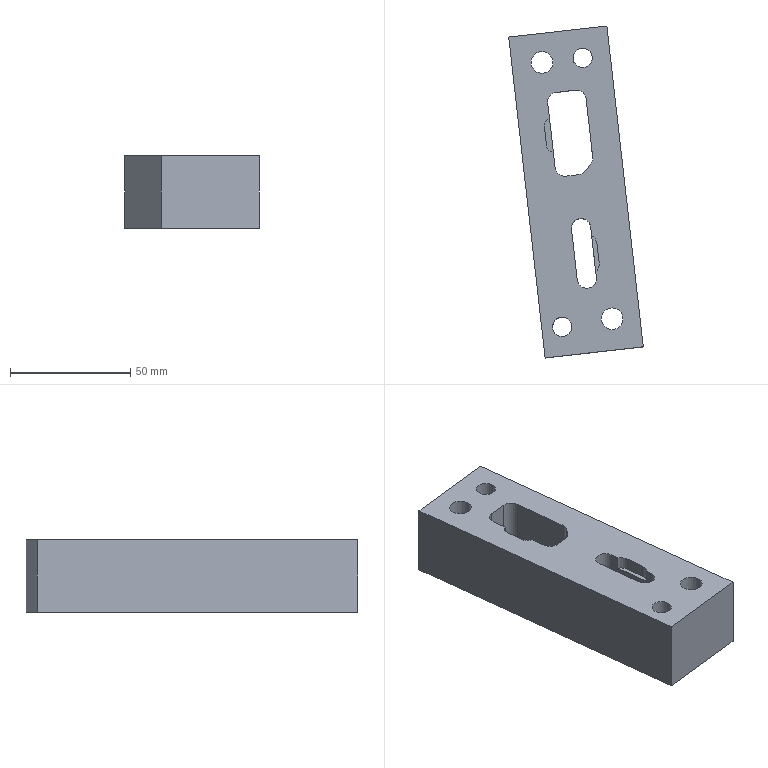Part | NX | features TB 2 | 1 solid | 40 faces | box 55.812 x 137.761 x 30 mm | volume 131881 mm3 | plane 21 | cylinder 19 | commonest cylinder face diameters 8 x7 9 x4 6 x2 8.001 x2 8.5 x2 14.5 x2
STEP:
#1=CARTESIAN_POINT('',(233.25,231.272,30.));
#2=VERTEX_POINT('',#1);
#3=CARTESIAN_POINT('',(233.502,229.054,30.));
#4=VERTEX_POINT('',#3);
#5=CARTESIAN_POINT('',(261.968,-22.421,30.));
#6=DIRECTION('',(0.1125,-0.9937,0.));
#7=VECTOR('',#6,1000.);
#8=LINE('',#5,#7);
#9=EDGE_CURVE('',#2,#4,#8,.T.);
#10=ORIENTED_EDGE('',*,*,#9,.T.);
#11=CARTESIAN_POINT('',(225.552,228.154,30.));
#12=VERTEX_POINT('',#11);
#13=CARTESIAN_POINT('',(229.527,228.604,30.));
#14=DIRECTION('',(0.,0.,1.));
#15=DIRECTION('',(0.,-1.,0.));
#16=AXIS2_PLACEMENT_3D('',#13,#14,#15);
#17=CIRCLE('',#16,4.);
#18=EDGE_CURVE('',#12,#4,#17,.T.);
#19=ORIENTED_EDGE('',*,*,#18,.F.);
#20=CARTESIAN_POINT('',(223.19,249.026,30.));
#21=VERTEX_POINT('',#20);
#22=CARTESIAN_POINT('',(254.019,-23.321,30.));
#23=DIRECTION('',(0.1125,-0.9937,0.));
#24=VECTOR('',#23,1000.);
#25=LINE('',#22,#24);
#26=EDGE_CURVE('',#21,#12,#25,.T.);
#27=ORIENTED_EDGE('',*,*,#26,.F.);
#28=CARTESIAN_POINT('',(231.139,249.926,30.));
#29=VERTEX_POINT('',#28);
#30=CARTESIAN_POINT('',(227.164,249.476,30.));
#31=DIRECTION('',(0.,0.,1.));
#32=DIRECTION('',(0.,-1.,0.));
#33=AXIS2_PLACEMENT_3D('',#30,#31,#32);
#34=CIRCLE('',#33,4.);
#35=EDGE_CURVE('',#29,#21,#34,.T.);
#36=ORIENTED_EDGE('',*,*,#35,.F.);
#37=CARTESIAN_POINT('',(231.527,246.496,30.));
#38=VERTEX_POINT('',#37);
#39=CARTESIAN_POINT('',(261.968,-22.421,30.));
#40=DIRECTION('',(0.1125,-0.9937,0.));
#41=VECTOR('',#40,1000.);
#42=LINE('',#39,#41);
#43=EDGE_CURVE('',#29,#38,#42,.T.);
#44=ORIENTED_EDGE('',*,*,#43,.T.);
#45=CARTESIAN_POINT('',(233.736,243.112,30.));
#46=VERTEX_POINT('',#45);
#47=CARTESIAN_POINT('',(229.265,242.606,30.));
#48=DIRECTION('',(0.,0.,-1.));
#49=DIRECTION('',(0.,-1.,0.));
#50=AXIS2_PLACEMENT_3D('',#47,#48,#49);
#51=CIRCLE('',#50,4.5);
#52=EDGE_CURVE('',#38,#46,#51,.T.);
#53=ORIENTED_EDGE('',*,*,#52,.T.);
#54=CARTESIAN_POINT('',(234.647,235.064,30.));
#55=VERTEX_POINT('',#54);
#56=CARTESIAN_POINT('',(234.372,237.498,30.));
#57=DIRECTION('',(0.1125,-0.9937,0.));
#58=VECTOR('',#57,1000.);
#59=LINE('',#56,#58);
#60=EDGE_CURVE('',#46,#55,#59,.T.);
#61=ORIENTED_EDGE('',*,*,#60,.T.);
#62=CARTESIAN_POINT('',(230.176,234.558,30.));
#63=DIRECTION('',(0.,0.,-1.));
#64=DIRECTION('',(0.,-1.,0.));
#65=AXIS2_PLACEMENT_3D('',#62,#63,#64);
#66=CIRCLE('',#65,4.5);
#67=EDGE_CURVE('',#55,#2,#66,.T.);
#68=ORIENTED_EDGE('',*,*,#67,.T.);
#69=EDGE_LOOP('',(#10,#19,#27,#36,#44,#53,#61,#68));
#70=FACE_BOUND('',#69,.T.);
#71=CARTESIAN_POINT('',(237.879,333.435,30.));
#72=VERTEX_POINT('',#71);
#73=CARTESIAN_POINT('',(252.951,200.285,30.));
#74=VERTEX_POINT('',#73);
#75=CARTESIAN_POINT('',(214.764,537.629,30.));
#76=DIRECTION('',(0.1125,-0.9937,0.));
#77=VECTOR('',#76,1000.);
#78=LINE('',#75,#77);
#79=EDGE_CURVE('',#72,#74,#78,.T.);
#80=ORIENTED_EDGE('',*,*,#79,.F.);
#81=CARTESIAN_POINT('',(197.139,328.823,30.));
#82=VERTEX_POINT('',#81);
#83=CARTESIAN_POINT('',(443.385,356.698,30.));
#84=DIRECTION('',(0.9937,0.1125,0.));
#85=VECTOR('',#84,1000.);
#86=LINE('',#83,#85);
#87=EDGE_CURVE('',#82,#72,#86,.T.);
#88=ORIENTED_EDGE('',*,*,#87,.F.);
#89=CARTESIAN_POINT('',(212.211,195.673,30.));
#90=VERTEX_POINT('',#89);
#91=CARTESIAN_POINT('',(174.024,533.017,30.));
#92=DIRECTION('',(-0.1125,0.9937,0.));
#93=VECTOR('',#92,1000.);
#94=LINE('',#91,#93);
#95=EDGE_CURVE('',#90,#82,#94,.T.);
#96=ORIENTED_EDGE('',*,*,#95,.F.);
#97=CARTESIAN_POINT('',(458.458,223.548,30.));
#98=DIRECTION('',(-0.9937,-0.1125,0.));
#99=VECTOR('',#98,1000.);
#100=LINE('',#97,#99);
#101=EDGE_CURVE('',#74,#90,#100,.T.);
#102=ORIENTED_EDGE('',*,*,#101,.F.);
#103=EDGE_LOOP('',(#80,#88,#96,#102));
#104=FACE_BOUND('',#103,.T.);
#105=CARTESIAN_POINT('',(240.062,216.409,30.));
#106=VERTEX_POINT('',#105);
#107=CARTESIAN_POINT('',(240.062,211.909,30.));
#108=DIRECTION('',(0.,0.,-1.));
#109=DIRECTION('',(0.,1.,0.));
#110=AXIS2_PLACEMENT_3D('',#107,#108,#109);
#111=CIRCLE('',#110,4.5);
#112=EDGE_CURVE('',#106,#106,#111,.T.);
#113=ORIENTED_EDGE('',*,*,#112,.T.);
#114=EDGE_LOOP('',(#113));
#115=FACE_BOUND('',#114,.T.);
#116=CARTESIAN_POINT('',(210.909,322.805,30.));
#117=VERTEX_POINT('',#116);
#118=CARTESIAN_POINT('',(210.909,318.305,30.));
#119=DIRECTION('',(0.,0.,1.));
#120=DIRECTION('',(0.,1.,0.));
#121=AXIS2_PLACEMENT_3D('',#118,#119,#120);
#122=CIRCLE('',#121,4.5);
#123=EDGE_CURVE('',#117,#117,#122,.T.);
#124=ORIENTED_EDGE('',*,*,#123,.F.);
#125=EDGE_LOOP('',(#124));
#126=FACE_BOUND('',#125,.T.);
#127=CARTESIAN_POINT('',(215.619,281.141,30.));
#128=VERTEX_POINT('',#127);
#129=CARTESIAN_POINT('',(212.803,283.799,30.));
#130=VERTEX_POINT('',#129);
#131=CARTESIAN_POINT('',(215.783,284.137,30.));
#132=DIRECTION('',(0.,0.,-1.));
#133=DIRECTION('',(0.,-1.,0.));
#134=AXIS2_PLACEMENT_3D('',#131,#132,#133);
#135=CIRCLE('',#134,3.);
#136=EDGE_CURVE('',#128,#130,#135,.T.);
#137=ORIENTED_EDGE('',*,*,#136,.T.);
#138=CARTESIAN_POINT('',(211.903,291.748,30.));
#139=VERTEX_POINT('',#138);
#140=CARTESIAN_POINT('',(185.72,523.047,30.));
#141=DIRECTION('',(-0.1125,0.9937,0.));
#142=VECTOR('',#141,1000.);
#143=LINE('',#140,#142);
#144=EDGE_CURVE('',#130,#139,#143,.T.);
#145=ORIENTED_EDGE('',*,*,#144,.T.);
#146=CARTESIAN_POINT('',(214.054,294.969,30.));
#147=VERTEX_POINT('',#146);
#148=CARTESIAN_POINT('',(214.884,292.086,30.));
#149=DIRECTION('',(0.,0.,-1.));
#150=DIRECTION('',(0.,-1.,0.));
#151=AXIS2_PLACEMENT_3D('',#148,#149,#150);
#152=CIRCLE('',#151,3.);
#153=EDGE_CURVE('',#139,#147,#152,.T.);
#154=ORIENTED_EDGE('',*,*,#153,.T.);
#155=CARTESIAN_POINT('',(213.318,301.469,30.));
#156=VERTEX_POINT('',#155);
#157=CARTESIAN_POINT('',(186.942,534.48,30.));
#158=DIRECTION('',(0.1125,-0.9937,0.));
#159=VECTOR('',#158,1000.);
#160=LINE('',#157,#159);
#161=EDGE_CURVE('',#156,#147,#160,.T.);
#162=ORIENTED_EDGE('',*,*,#161,.F.);
#163=CARTESIAN_POINT('',(216.843,305.894,30.));
#164=VERTEX_POINT('',#163);
#165=CARTESIAN_POINT('',(217.293,301.919,30.));
#166=DIRECTION('',(0.,0.,1.));
#167=DIRECTION('',(0.,-1.,0.));
#168=AXIS2_PLACEMENT_3D('',#165,#166,#167);
#169=CIRCLE('',#168,4.);
#170=EDGE_CURVE('',#164,#156,#169,.T.);
#171=ORIENTED_EDGE('',*,*,#170,.F.);
#172=CARTESIAN_POINT('',(224.792,306.794,30.));
#173=VERTEX_POINT('',#172);
#174=CARTESIAN_POINT('',(453.153,332.644,30.));
#175=DIRECTION('',(0.9937,0.1125,0.));
#176=VECTOR('',#175,1000.);
#177=LINE('',#174,#176);
#178=EDGE_CURVE('',#164,#173,#177,.T.);
#179=ORIENTED_EDGE('',*,*,#178,.T.);
#180=CARTESIAN_POINT('',(229.217,303.269,30.));
#181=VERTEX_POINT('',#180);
#182=CARTESIAN_POINT('',(225.242,302.819,30.));
#183=DIRECTION('',(0.,0.,1.));
#184=DIRECTION('',(0.,-1.,0.));
#185=AXIS2_PLACEMENT_3D('',#182,#183,#184);
#186=CIRCLE('',#185,4.);
#187=EDGE_CURVE('',#181,#173,#186,.T.);
#188=ORIENTED_EDGE('',*,*,#187,.F.);
#189=CARTESIAN_POINT('',(231.955,279.08,30.));
#190=VERTEX_POINT('',#189);
#191=CARTESIAN_POINT('',(230.585,291.183,30.));
#192=DIRECTION('',(0.1125,-0.9937,0.));
#193=VECTOR('',#192,1000.);
#194=LINE('',#191,#193);
#195=EDGE_CURVE('',#181,#190,#194,.T.);
#196=ORIENTED_EDGE('',*,*,#195,.T.);
#197=CARTESIAN_POINT('',(231.109,276.138,30.));
#198=VERTEX_POINT('',#197);
#199=CARTESIAN_POINT('',(227.98,278.63,30.));
#200=DIRECTION('',(0.,0.,1.));
#201=DIRECTION('',(0.,-1.,0.));
#202=AXIS2_PLACEMENT_3D('',#199,#200,#201);
#203=CIRCLE('',#202,4.);
#204=EDGE_CURVE('',#198,#190,#203,.T.);
#205=ORIENTED_EDGE('',*,*,#204,.F.);
#206=CARTESIAN_POINT('',(228.768,273.199,30.));
#207=VERTEX_POINT('',#206);
#208=CARTESIAN_POINT('',(447.728,548.06,30.));
#209=DIRECTION('',(0.6231,0.7822,0.));
#210=VECTOR('',#209,1000.);
#211=LINE('',#208,#210);
#212=EDGE_CURVE('',#207,#198,#211,.T.);
#213=ORIENTED_EDGE('',*,*,#212,.F.);
#214=CARTESIAN_POINT('',(226.089,271.717,30.));
#215=VERTEX_POINT('',#214);
#216=CARTESIAN_POINT('',(225.639,275.692,30.));
#217=DIRECTION('',(0.,0.,1.));
#218=DIRECTION('',(0.,-1.,0.));
#219=AXIS2_PLACEMENT_3D('',#216,#217,#218);
#220=CIRCLE('',#219,4.);
#221=EDGE_CURVE('',#215,#207,#220,.T.);
#222=ORIENTED_EDGE('',*,*,#221,.F.);
#223=CARTESIAN_POINT('',(220.78,271.116,30.));
#224=VERTEX_POINT('',#223);
#225=CARTESIAN_POINT('',(457.09,297.866,30.));
#226=DIRECTION('',(0.9937,0.1125,0.));
#227=VECTOR('',#226,1000.);
#228=LINE('',#225,#227);
#229=EDGE_CURVE('',#224,#215,#228,.T.);
#230=ORIENTED_EDGE('',*,*,#229,.F.);
#231=CARTESIAN_POINT('',(216.355,274.641,30.));
#232=VERTEX_POINT('',#231);
#233=CARTESIAN_POINT('',(220.33,275.091,30.));
#234=DIRECTION('',(0.,0.,1.));
#235=DIRECTION('',(0.,-1.,0.));
#236=AXIS2_PLACEMENT_3D('',#233,#234,#235);
#237=CIRCLE('',#236,4.);
#238=EDGE_CURVE('',#232,#224,#237,.T.);
#239=ORIENTED_EDGE('',*,*,#238,.F.);
#240=CARTESIAN_POINT('',(186.942,534.48,30.));
#241=DIRECTION('',(0.1125,-0.9937,0.));
#242=VECTOR('',#241,1000.);
#243=LINE('',#240,#242);
#244=EDGE_CURVE('',#128,#232,#243,.T.);
#245=ORIENTED_EDGE('',*,*,#244,.F.);
#246=EDGE_LOOP('',(#137,#145,#154,#162,#171,#179,#188,#196,#205,#213,#222,#230,#239,#245));
#247=FACE_BOUND('',#246,.T.);
#248=CARTESIAN_POINT('',(223.801,320.217,30.));
#249=VERTEX_POINT('',#248);
#250=CARTESIAN_POINT('',(227.801,320.217,30.));
#251=DIRECTION('',(0.,0.,1.));
#252=DIRECTION('',(-1.,0.,0.));
#253=AXIS2_PLACEMENT_3D('',#250,#251,#252);
#254=CIRCLE('',#253,4.);
#255=EDGE_CURVE('',#249,#249,#254,.T.);
#256=ORIENTED_EDGE('',*,*,#255,.F.);
#257=EDGE_LOOP('',(#256));
#258=FACE_BOUND('',#257,.T.);
#259=CARTESIAN_POINT('',(223.308,208.553,30.));
#260=VERTEX_POINT('',#259);
#261=CARTESIAN_POINT('',(219.308,208.553,30.));
#262=DIRECTION('',(0.,0.,-1.));
#263=DIRECTION('',(1.,0.,0.));
#264=AXIS2_PLACEMENT_3D('',#261,#262,#263);
#265=CIRCLE('',#264,4.);
#266=EDGE_CURVE('',#260,#260,#265,.T.);
#267=ORIENTED_EDGE('',*,*,#266,.T.);
#268=EDGE_LOOP('',(#267));
#269=FACE_BOUND('',#268,.T.);
#270=CARTESIAN_POINT('',(427.226,561.68,30.));
#271=DIRECTION('',(0.,0.,-1.));
#272=DIRECTION('',(-0.9981,0.06177,0.));
#273=AXIS2_PLACEMENT_3D('',#270,#271,#272);
#274=PLANE('',#273);
#275=ADVANCED_FACE('',(#70,#104,#115,#126,#247,#258,#269),#274,.F.);
#276=CARTESIAN_POINT('',(219.308,204.303,0.));
#277=VERTEX_POINT('',#276);
#278=CARTESIAN_POINT('',(219.308,208.553,0.));
#279=DIRECTION('',(0.,0.,1.));
#280=DIRECTION('',(0.,-1.,0.));
#281=AXIS2_PLACEMENT_3D('',#278,#279,#280);
#282=CIRCLE('',#281,4.25);
#283=EDGE_CURVE('',#277,#277,#282,.T.);
#284=ORIENTED_EDGE('',*,*,#283,.T.);
#285=EDGE_LOOP('',(#284));
#286=FACE_BOUND('',#285,.T.);
#287=CARTESIAN_POINT('',(227.801,315.967,0.));
#288=VERTEX_POINT('',#287);
#289=CARTESIAN_POINT('',(227.801,320.217,0.));
#290=DIRECTION('',(0.,0.,1.));
#291=DIRECTION('',(0.,-1.,0.));
#292=AXIS2_PLACEMENT_3D('',#289,#290,#291);
#293=CIRCLE('',#292,4.25);
#294=EDGE_CURVE('',#288,#288,#293,.T.);
#295=ORIENTED_EDGE('',*,*,#294,.T.);
#296=EDGE_LOOP('',(#295));
#297=FACE_BOUND('',#296,.T.);
#298=CARTESIAN_POINT('',(231.955,279.08,0.));
#299=VERTEX_POINT('',#298);
#300=CARTESIAN_POINT('',(229.217,303.269,0.));
#301=VERTEX_POINT('',#300);
#302=CARTESIAN_POINT('',(230.585,291.183,0.));
#303=DIRECTION('',(-0.1125,0.9937,0.));
#304=VECTOR('',#303,1000.);
#305=LINE('',#302,#304);
#306=EDGE_CURVE('',#299,#301,#305,.T.);
#307=ORIENTED_EDGE('',*,*,#306,.T.);
#308=CARTESIAN_POINT('',(224.792,306.794,0.));
#309=VERTEX_POINT('',#308);
#310=CARTESIAN_POINT('',(225.242,302.819,0.));
#311=DIRECTION('',(0.,0.,-1.));
#312=DIRECTION('',(0.,-1.,0.));
#313=AXIS2_PLACEMENT_3D('',#310,#311,#312);
#314=CIRCLE('',#313,4.);
#315=EDGE_CURVE('',#309,#301,#314,.T.);
#316=ORIENTED_EDGE('',*,*,#315,.F.);
#317=CARTESIAN_POINT('',(216.843,305.894,0.));
#318=VERTEX_POINT('',#317);
#319=CARTESIAN_POINT('',(453.153,332.644,0.));
#320=DIRECTION('',(-0.9937,-0.1125,0.));
#321=VECTOR('',#320,1000.);
#322=LINE('',#319,#321);
#323=EDGE_CURVE('',#309,#318,#322,.T.);
#324=ORIENTED_EDGE('',*,*,#323,.T.);
#325=CARTESIAN_POINT('',(213.318,301.469,0.));
#326=VERTEX_POINT('',#325);
#327=CARTESIAN_POINT('',(217.293,301.919,0.));
#328=DIRECTION('',(0.,0.,-1.));
#329=DIRECTION('',(0.,-1.,0.));
#330=AXIS2_PLACEMENT_3D('',#327,#328,#329);
#331=CIRCLE('',#330,4.);
#332=EDGE_CURVE('',#326,#318,#331,.T.);
#333=ORIENTED_EDGE('',*,*,#332,.F.);
#334=CARTESIAN_POINT('',(216.355,274.641,0.));
#335=VERTEX_POINT('',#334);
#336=CARTESIAN_POINT('',(214.837,288.055,0.));
#337=DIRECTION('',(0.1125,-0.9937,0.));
#338=VECTOR('',#337,1000.);
#339=LINE('',#336,#338);
#340=EDGE_CURVE('',#326,#335,#339,.T.);
#341=ORIENTED_EDGE('',*,*,#340,.T.);
#342=CARTESIAN_POINT('',(220.78,271.116,0.));
#343=VERTEX_POINT('',#342);
#344=CARTESIAN_POINT('',(220.33,275.091,0.));
#345=DIRECTION('',(0.,0.,-1.));
#346=DIRECTION('',(0.,-1.,0.));
#347=AXIS2_PLACEMENT_3D('',#344,#345,#346);
#348=CIRCLE('',#347,4.);
#349=EDGE_CURVE('',#343,#335,#348,.T.);
#350=ORIENTED_EDGE('',*,*,#349,.F.);
#351=CARTESIAN_POINT('',(226.089,271.717,0.));
#352=VERTEX_POINT('',#351);
#353=CARTESIAN_POINT('',(457.09,297.866,0.));
#354=DIRECTION('',(-0.9937,-0.1125,0.));
#355=VECTOR('',#354,1000.);
#356=LINE('',#353,#355);
#357=EDGE_CURVE('',#352,#343,#356,.T.);
#358=ORIENTED_EDGE('',*,*,#357,.F.);
#359=CARTESIAN_POINT('',(228.768,273.199,0.));
#360=VERTEX_POINT('',#359);
#361=CARTESIAN_POINT('',(225.639,275.692,0.));
#362=DIRECTION('',(0.,0.,-1.));
#363=DIRECTION('',(0.,-1.,0.));
#364=AXIS2_PLACEMENT_3D('',#361,#362,#363);
#365=CIRCLE('',#364,4.);
#366=EDGE_CURVE('',#360,#352,#365,.T.);
#367=ORIENTED_EDGE('',*,*,#366,.F.);
#368=CARTESIAN_POINT('',(231.109,276.138,0.));
#369=VERTEX_POINT('',#368);
#370=CARTESIAN_POINT('',(447.728,548.06,0.));
#371=DIRECTION('',(-0.6231,-0.7822,0.));
#372=VECTOR('',#371,1000.);
#373=LINE('',#370,#372);
#374=EDGE_CURVE('',#369,#360,#373,.T.);
#375=ORIENTED_EDGE('',*,*,#374,.F.);
#376=CARTESIAN_POINT('',(227.98,278.63,0.));
#377=DIRECTION('',(0.,0.,-1.));
#378=DIRECTION('',(0.,-1.,0.));
#379=AXIS2_PLACEMENT_3D('',#376,#377,#378);
#380=CIRCLE('',#379,4.);
#381=EDGE_CURVE('',#299,#369,#380,.T.);
#382=ORIENTED_EDGE('',*,*,#381,.F.);
#383=EDGE_LOOP('',(#307,#316,#324,#333,#341,#350,#358,#367,#375,#382));
#384=FACE_BOUND('',#383,.T.);
#385=CARTESIAN_POINT('',(231.139,249.926,0.));
#386=VERTEX_POINT('',#385);
#387=CARTESIAN_POINT('',(233.502,229.054,0.));
#388=VERTEX_POINT('',#387);
#389=CARTESIAN_POINT('',(261.968,-22.421,0.));
#390=DIRECTION('',(0.1125,-0.9937,0.));
#391=VECTOR('',#390,1000.);
#392=LINE('',#389,#391);
#393=EDGE_CURVE('',#386,#388,#392,.T.);
#394=ORIENTED_EDGE('',*,*,#393,.F.);
#395=CARTESIAN_POINT('',(223.19,249.026,0.));
#396=VERTEX_POINT('',#395);
#397=CARTESIAN_POINT('',(227.164,249.476,0.));
#398=DIRECTION('',(0.,0.,-1.));
#399=DIRECTION('',(0.,-1.,0.));
#400=AXIS2_PLACEMENT_3D('',#397,#398,#399);
#401=CIRCLE('',#400,4.);
#402=EDGE_CURVE('',#396,#386,#401,.T.);
#403=ORIENTED_EDGE('',*,*,#402,.F.);
#404=CARTESIAN_POINT('',(225.552,228.154,0.));
#405=VERTEX_POINT('',#404);
#406=CARTESIAN_POINT('',(225.777,226.166,0.));
#407=DIRECTION('',(-0.1125,0.9937,0.));
#408=VECTOR('',#407,1000.);
#409=LINE('',#406,#408);
#410=EDGE_CURVE('',#405,#396,#409,.T.);
#411=ORIENTED_EDGE('',*,*,#410,.F.);
#412=CARTESIAN_POINT('',(229.527,228.604,0.));
#413=DIRECTION('',(0.,0.,-1.));
#414=DIRECTION('',(0.,-1.,0.));
#415=AXIS2_PLACEMENT_3D('',#412,#413,#414);
#416=CIRCLE('',#415,4.);
#417=EDGE_CURVE('',#388,#405,#416,.T.);
#418=ORIENTED_EDGE('',*,*,#417,.F.);
#419=EDGE_LOOP('',(#394,#403,#411,#418));
#420=FACE_BOUND('',#419,.T.);
#421=CARTESIAN_POINT('',(210.909,325.555,0.));
#422=VERTEX_POINT('',#421);
#423=CARTESIAN_POINT('',(210.909,318.305,0.));
#424=DIRECTION('',(0.,0.,1.));
#425=DIRECTION('',(0.,1.,0.));
#426=AXIS2_PLACEMENT_3D('',#423,#424,#425);
#427=CIRCLE('',#426,7.25);
#428=EDGE_CURVE('',#422,#422,#427,.T.);
#429=ORIENTED_EDGE('',*,*,#428,.T.);
#430=EDGE_LOOP('',(#429));
#431=FACE_BOUND('',#430,.T.);
#432=CARTESIAN_POINT('',(240.062,219.159,0.));
#433=VERTEX_POINT('',#432);
#434=CARTESIAN_POINT('',(240.062,211.909,0.));
#435=DIRECTION('',(0.,0.,-1.));
#436=DIRECTION('',(0.,1.,0.));
#437=AXIS2_PLACEMENT_3D('',#434,#435,#436);
#438=CIRCLE('',#437,7.25);
#439=EDGE_CURVE('',#433,#433,#438,.T.);
#440=ORIENTED_EDGE('',*,*,#439,.F.);
#441=EDGE_LOOP('',(#440));
#442=FACE_BOUND('',#441,.T.);
#443=CARTESIAN_POINT('',(197.139,328.823,0.));
#444=VERTEX_POINT('',#443);
#445=CARTESIAN_POINT('',(237.879,333.435,0.));
#446=VERTEX_POINT('',#445);
#447=CARTESIAN_POINT('',(443.385,356.698,0.));
#448=DIRECTION('',(0.9937,0.1125,0.));
#449=VECTOR('',#448,1000.);
#450=LINE('',#447,#449);
#451=EDGE_CURVE('',#444,#446,#450,.T.);
#452=ORIENTED_EDGE('',*,*,#451,.T.);
#453=CARTESIAN_POINT('',(252.951,200.285,0.));
#454=VERTEX_POINT('',#453);
#455=CARTESIAN_POINT('',(214.764,537.629,0.));
#456=DIRECTION('',(0.1125,-0.9937,0.));
#457=VECTOR('',#456,1000.);
#458=LINE('',#455,#457);
#459=EDGE_CURVE('',#446,#454,#458,.T.);
#460=ORIENTED_EDGE('',*,*,#459,.T.);
#461=CARTESIAN_POINT('',(212.211,195.673,0.));
#462=VERTEX_POINT('',#461);
#463=CARTESIAN_POINT('',(458.458,223.548,0.));
#464=DIRECTION('',(-0.9937,-0.1125,0.));
#465=VECTOR('',#464,1000.);
#466=LINE('',#463,#465);
#467=EDGE_CURVE('',#454,#462,#466,.T.);
#468=ORIENTED_EDGE('',*,*,#467,.T.);
#469=CARTESIAN_POINT('',(174.024,533.017,0.));
#470=DIRECTION('',(-0.1125,0.9937,0.));
#471=VECTOR('',#470,1000.);
#472=LINE('',#469,#471);
#473=EDGE_CURVE('',#462,#444,#472,.T.);
#474=ORIENTED_EDGE('',*,*,#473,.T.);
#475=EDGE_LOOP('',(#452,#460,#468,#474));
#476=FACE_BOUND('',#475,.T.);
#477=CARTESIAN_POINT('',(420.271,560.892,0.));
#478=DIRECTION('',(0.,0.,-1.));
#479=DIRECTION('',(-0.9981,0.06177,0.));
#480=AXIS2_PLACEMENT_3D('',#477,#478,#479);
#481=PLANE('',#480);
#482=ADVANCED_FACE('',(#286,#297,#384,#420,#431,#442,#476),#481,.T.);
#483=CARTESIAN_POINT('',(233.25,231.272,24.8));
#484=VERTEX_POINT('',#483);
#485=CARTESIAN_POINT('',(234.647,235.064,24.8));
#486=VERTEX_POINT('',#485);
#487=CARTESIAN_POINT('',(230.176,234.558,24.8));
#488=DIRECTION('',(0.,0.,1.));
#489=DIRECTION('',(0.,1.,0.));
#490=AXIS2_PLACEMENT_3D('',#487,#488,#489);
#491=CIRCLE('',#490,4.5);
#492=EDGE_CURVE('',#484,#486,#491,.T.);
#493=ORIENTED_EDGE('',*,*,#492,.T.);
#494=CARTESIAN_POINT('',(233.736,243.112,24.8));
#495=VERTEX_POINT('',#494);
#496=CARTESIAN_POINT('',(234.372,237.498,24.8));
#497=DIRECTION('',(0.1125,-0.9937,0.));
#498=VECTOR('',#497,1000.);
#499=LINE('',#496,#498);
#500=EDGE_CURVE('',#495,#486,#499,.T.);
#501=ORIENTED_EDGE('',*,*,#500,.F.);
#502=CARTESIAN_POINT('',(231.527,246.496,24.8));
#503=VERTEX_POINT('',#502);
#504=CARTESIAN_POINT('',(229.265,242.606,24.8));
#505=DIRECTION('',(0.,0.,1.));
#506=DIRECTION('',(0.,1.,0.));
#507=AXIS2_PLACEMENT_3D('',#504,#505,#506);
#508=CIRCLE('',#507,4.5);
#509=EDGE_CURVE('',#495,#503,#508,.T.);
#510=ORIENTED_EDGE('',*,*,#509,.T.);
#511=CARTESIAN_POINT('',(233.727,227.066,24.8));
#512=DIRECTION('',(-0.1125,0.9937,0.));
#513=VECTOR('',#512,1000.);
#514=LINE('',#511,#513);
#515=EDGE_CURVE('',#484,#503,#514,.T.);
#516=ORIENTED_EDGE('',*,*,#515,.F.);
#517=EDGE_LOOP('',(#493,#501,#510,#516));
#518=FACE_BOUND('',#517,.T.);
#519=CARTESIAN_POINT('',(223.64,236.283,24.8));
#520=DIRECTION('',(0.,0.,-1.));
#521=DIRECTION('',(-0.9981,0.06177,0.));
#522=AXIS2_PLACEMENT_3D('',#519,#520,#521);
#523=PLANE('',#522);
#524=ADVANCED_FACE('',(#518),#523,.F.);
#525=ORIENTED_EDGE('',*,*,#509,.F.);
#526=CARTESIAN_POINT('',(233.736,243.112,25.7));
#527=DIRECTION('',(0.,0.,-1.));
#528=VECTOR('',#527,1000.);
#529=LINE('',#526,#528);
#530=EDGE_CURVE('',#46,#495,#529,.T.);
#531=ORIENTED_EDGE('',*,*,#530,.F.);
#532=ORIENTED_EDGE('',*,*,#52,.F.);
#533=CARTESIAN_POINT('',(231.527,246.496,25.7));
#534=DIRECTION('',(0.,0.,1.));
#535=VECTOR('',#534,1000.);
#536=LINE('',#533,#535);
#537=EDGE_CURVE('',#503,#38,#536,.T.);
#538=ORIENTED_EDGE('',*,*,#537,.F.);
#539=EDGE_LOOP('',(#525,#531,#532,#538));
#540=FACE_BOUND('',#539,.T.);
#541=CARTESIAN_POINT('',(229.265,242.606,25.7));
#542=DIRECTION('',(0.,0.,1.));
#543=DIRECTION('',(0.9981,-0.06177,0.));
#544=AXIS2_PLACEMENT_3D('',#541,#542,#543);
#545=CYLINDRICAL_SURFACE('',#544,4.5);
#546=ADVANCED_FACE('',(#540),#545,.F.);
#547=ORIENTED_EDGE('',*,*,#67,.F.);
#548=CARTESIAN_POINT('',(234.647,235.064,25.7));
#549=DIRECTION('',(0.,0.,1.));
#550=VECTOR('',#549,1000.);
#551=LINE('',#548,#550);
#552=EDGE_CURVE('',#486,#55,#551,.T.);
#553=ORIENTED_EDGE('',*,*,#552,.F.);
#554=ORIENTED_EDGE('',*,*,#492,.F.);
#555=CARTESIAN_POINT('',(233.25,231.272,25.7));
#556=DIRECTION('',(0.,0.,-1.));
#557=VECTOR('',#556,1000.);
#558=LINE('',#555,#557);
#559=EDGE_CURVE('',#2,#484,#558,.T.);
#560=ORIENTED_EDGE('',*,*,#559,.F.);
#561=EDGE_LOOP('',(#547,#553,#554,#560));
#562=FACE_BOUND('',#561,.T.);
#563=CARTESIAN_POINT('',(230.176,234.558,25.7));
#564=DIRECTION('',(0.,0.,1.));
#565=DIRECTION('',(0.9981,-0.06177,0.));
#566=AXIS2_PLACEMENT_3D('',#563,#564,#565);
#567=CYLINDRICAL_SURFACE('',#566,4.5);
#568=ADVANCED_FACE('',(#562),#567,.F.);
#569=CARTESIAN_POINT('',(215.619,281.141,24.8));
#570=VERTEX_POINT('',#569);
#571=CARTESIAN_POINT('',(214.054,294.969,24.8));
#572=VERTEX_POINT('',#571);
#573=CARTESIAN_POINT('',(213.993,295.507,24.8));
#574=DIRECTION('',(-0.1125,0.9937,0.));
#575=VECTOR('',#574,1000.);
#576=LINE('',#573,#575);
#577=EDGE_CURVE('',#570,#572,#576,.T.);
#578=ORIENTED_EDGE('',*,*,#577,.T.);
#579=CARTESIAN_POINT('',(211.903,291.748,24.8));
#580=VERTEX_POINT('',#579);
#581=CARTESIAN_POINT('',(214.884,292.086,24.8));
#582=DIRECTION('',(0.,0.,1.));
#583=DIRECTION('',(-0.9981,0.06177,0.));
#584=AXIS2_PLACEMENT_3D('',#581,#582,#583);
#585=CIRCLE('',#584,3.);
#586=EDGE_CURVE('',#572,#580,#585,.T.);
#587=ORIENTED_EDGE('',*,*,#586,.T.);
#588=CARTESIAN_POINT('',(212.803,283.799,24.8));
#589=VERTEX_POINT('',#588);
#590=CARTESIAN_POINT('',(185.72,523.047,24.8));
#591=DIRECTION('',(-0.1125,0.9937,0.));
#592=VECTOR('',#591,1000.);
#593=LINE('',#590,#592);
#594=EDGE_CURVE('',#589,#580,#593,.T.);
#595=ORIENTED_EDGE('',*,*,#594,.F.);
#596=CARTESIAN_POINT('',(215.783,284.137,24.8));
#597=DIRECTION('',(0.,0.,1.));
#598=DIRECTION('',(-0.9981,0.06177,0.));
#599=AXIS2_PLACEMENT_3D('',#596,#597,#598);
#600=CIRCLE('',#599,3.);
#601=EDGE_CURVE('',#589,#570,#600,.T.);
#602=ORIENTED_EDGE('',*,*,#601,.T.);
#603=EDGE_LOOP('',(#578,#587,#595,#602));
#604=FACE_BOUND('',#603,.T.);
#605=CARTESIAN_POINT('',(213.496,295.451,24.8));
#606=DIRECTION('',(0.,0.,1.));
#607=DIRECTION('',(-0.9981,0.06177,0.));
#608=AXIS2_PLACEMENT_3D('',#605,#606,#607);
#609=PLANE('',#608);
#610=ADVANCED_FACE('',(#604),#609,.T.);
#611=CARTESIAN_POINT('',(240.062,219.159,15.));
#612=VERTEX_POINT('',#611);
#613=CARTESIAN_POINT('',(240.062,211.909,15.));
#614=DIRECTION('',(0.,0.,1.));
#615=DIRECTION('',(0.,1.,0.));
#616=AXIS2_PLACEMENT_3D('',#613,#614,#615);
#617=CIRCLE('',#616,7.25);
#618=EDGE_CURVE('',#612,#612,#617,.T.);
#619=ORIENTED_EDGE('',*,*,#618,.F.);
#620=EDGE_LOOP('',(#619));
#621=FACE_BOUND('',#620,.T.);
#622=CARTESIAN_POINT('',(240.062,216.409,15.));
#623=VERTEX_POINT('',#622);
#624=CARTESIAN_POINT('',(240.062,211.909,15.));
#625=DIRECTION('',(0.,0.,-1.));
#626=DIRECTION('',(0.,1.,0.));
#627=AXIS2_PLACEMENT_3D('',#624,#625,#626);
#628=CIRCLE('',#627,4.5);
#629=EDGE_CURVE('',#623,#623,#628,.T.);
#630=ORIENTED_EDGE('',*,*,#629,.F.);
#631=EDGE_LOOP('',(#630));
#632=FACE_BOUND('',#631,.T.);
#633=CARTESIAN_POINT('',(220.808,284.202,15.));
#634=DIRECTION('',(0.,0.,-1.));
#635=DIRECTION('',(0.9981,-0.06177,0.));
#636=AXIS2_PLACEMENT_3D('',#633,#634,#635);
#637=PLANE('',#636);
#638=ADVANCED_FACE('',(#621,#632),#637,.T.);
#639=CARTESIAN_POINT('',(210.909,322.805,15.));
#640=VERTEX_POINT('',#639);
#641=CARTESIAN_POINT('',(210.909,318.305,15.));
#642=DIRECTION('',(0.,0.,1.));
#643=DIRECTION('',(0.,1.,0.));
#644=AXIS2_PLACEMENT_3D('',#641,#642,#643);
#645=CIRCLE('',#644,4.5);
#646=EDGE_CURVE('',#640,#640,#645,.T.);
#647=ORIENTED_EDGE('',*,*,#646,.T.);
#648=EDGE_LOOP('',(#647));
#649=FACE_BOUND('',#648,.T.);
#650=CARTESIAN_POINT('',(210.909,325.555,15.));
#651=VERTEX_POINT('',#650);
#652=CARTESIAN_POINT('',(210.909,318.305,15.));
#653=DIRECTION('',(0.,0.,-1.));
#654=DIRECTION('',(0.,1.,0.));
#655=AXIS2_PLACEMENT_3D('',#652,#653,#654);
#656=CIRCLE('',#655,7.25);
#657=EDGE_CURVE('',#651,#651,#656,.T.);
#658=ORIENTED_EDGE('',*,*,#657,.T.);
#659=EDGE_LOOP('',(#658));
#660=FACE_BOUND('',#659,.T.);
#661=CARTESIAN_POINT('',(220.808,284.202,15.));
#662=DIRECTION('',(0.,0.,-1.));
#663=DIRECTION('',(0.9981,-0.06177,0.));
#664=AXIS2_PLACEMENT_3D('',#661,#662,#663);
#665=PLANE('',#664);
#666=ADVANCED_FACE('',(#649,#660),#665,.T.);
#667=ORIENTED_EDGE('',*,*,#123,.T.);
#668=EDGE_LOOP('',(#667));
#669=FACE_BOUND('',#668,.T.);
#670=ORIENTED_EDGE('',*,*,#646,.F.);
#671=EDGE_LOOP('',(#670));
#672=FACE_BOUND('',#671,.T.);
#673=CARTESIAN_POINT('',(210.909,318.305,15.));
#674=DIRECTION('',(0.,0.,1.));
#675=DIRECTION('',(-0.9981,0.06177,0.));
#676=AXIS2_PLACEMENT_3D('',#673,#674,#675);
#677=CYLINDRICAL_SURFACE('',#676,4.5);
#678=ADVANCED_FACE('',(#669,#672),#677,.F.);
#679=ORIENTED_EDGE('',*,*,#112,.F.);
#680=EDGE_LOOP('',(#679));
#681=FACE_BOUND('',#680,.T.);
#682=ORIENTED_EDGE('',*,*,#629,.T.);
#683=EDGE_LOOP('',(#682));
#684=FACE_BOUND('',#683,.T.);
#685=CARTESIAN_POINT('',(240.062,211.909,15.));
#686=DIRECTION('',(0.,0.,-1.));
#687=DIRECTION('',(0.9981,-0.06177,0.));
#688=AXIS2_PLACEMENT_3D('',#685,#686,#687);
#689=CYLINDRICAL_SURFACE('',#688,4.5);
#690=ADVANCED_FACE('',(#681,#684),#689,.F.);
#691=ORIENTED_EDGE('',*,*,#153,.F.);
#692=CARTESIAN_POINT('',(211.903,291.748,14.5));
#693=DIRECTION('',(0.,0.,1.));
#694=VECTOR('',#693,1000.);
#695=LINE('',#692,#694);
#696=EDGE_CURVE('',#580,#139,#695,.T.);
#697=ORIENTED_EDGE('',*,*,#696,.F.);
#698=ORIENTED_EDGE('',*,*,#586,.F.);
#699=CARTESIAN_POINT('',(214.054,294.969,14.5));
#700=DIRECTION('',(0.,0.,-1.));
#701=VECTOR('',#700,1000.);
#702=LINE('',#699,#701);
#703=EDGE_CURVE('',#147,#572,#702,.T.);
#704=ORIENTED_EDGE('',*,*,#703,.F.);
#705=EDGE_LOOP('',(#691,#697,#698,#704));
#706=FACE_BOUND('',#705,.T.);
#707=CARTESIAN_POINT('',(214.884,292.086,14.5));
#708=DIRECTION('',(0.,0.,1.));
#709=DIRECTION('',(-0.9981,0.06177,0.));
#710=AXIS2_PLACEMENT_3D('',#707,#708,#709);
#711=CYLINDRICAL_SURFACE('',#710,3.);
#712=ADVANCED_FACE('',(#706),#711,.F.);
#713=ORIENTED_EDGE('',*,*,#594,.T.);
#714=ORIENTED_EDGE('',*,*,#696,.T.);
#715=ORIENTED_EDGE('',*,*,#144,.F.);
#716=CARTESIAN_POINT('',(212.803,283.799,14.5));
#717=DIRECTION('',(0.,0.,-1.));
#718=VECTOR('',#717,1000.);
#719=LINE('',#716,#718);
#720=EDGE_CURVE('',#130,#589,#719,.T.);
#721=ORIENTED_EDGE('',*,*,#720,.T.);
#722=EDGE_LOOP('',(#713,#714,#715,#721));
#723=FACE_BOUND('',#722,.T.);
#724=CARTESIAN_POINT('',(185.72,523.047,14.5));
#725=DIRECTION('',(-0.9937,-0.1125,0.));
#726=DIRECTION('',(0.1125,-0.9937,0.));
#727=AXIS2_PLACEMENT_3D('',#724,#725,#726);
#728=PLANE('',#727);
#729=ADVANCED_FACE('',(#723),#728,.F.);
#730=ORIENTED_EDGE('',*,*,#601,.F.);
#731=ORIENTED_EDGE('',*,*,#720,.F.);
#732=ORIENTED_EDGE('',*,*,#136,.F.);
#733=CARTESIAN_POINT('',(215.619,281.141,14.5));
#734=DIRECTION('',(0.,0.,1.));
#735=VECTOR('',#734,1000.);
#736=LINE('',#733,#735);
#737=EDGE_CURVE('',#570,#128,#736,.T.);
#738=ORIENTED_EDGE('',*,*,#737,.F.);
#739=EDGE_LOOP('',(#730,#731,#732,#738));
#740=FACE_BOUND('',#739,.T.);
#741=CARTESIAN_POINT('',(215.783,284.137,14.5));
#742=DIRECTION('',(0.,0.,-1.));
#743=DIRECTION('',(0.9981,-0.06177,0.));
#744=AXIS2_PLACEMENT_3D('',#741,#742,#743);
#745=CYLINDRICAL_SURFACE('',#744,3.);
#746=ADVANCED_FACE('',(#740),#745,.F.);
#747=ORIENTED_EDGE('',*,*,#95,.T.);
#748=CARTESIAN_POINT('',(197.139,328.823,0.));
#749=DIRECTION('',(0.,0.,1.));
#750=VECTOR('',#749,1000.);
#751=LINE('',#748,#750);
#752=EDGE_CURVE('',#444,#82,#751,.T.);
#753=ORIENTED_EDGE('',*,*,#752,.F.);
#754=ORIENTED_EDGE('',*,*,#473,.F.);
#755=CARTESIAN_POINT('',(212.211,195.673,0.));
#756=DIRECTION('',(0.,0.,1.));
#757=VECTOR('',#756,1000.);
#758=LINE('',#755,#757);
#759=EDGE_CURVE('',#462,#90,#758,.T.);
#760=ORIENTED_EDGE('',*,*,#759,.T.);
#761=EDGE_LOOP('',(#747,#753,#754,#760));
#762=FACE_BOUND('',#761,.T.);
#763=CARTESIAN_POINT('',(174.024,533.017,0.));
#764=DIRECTION('',(-0.9937,-0.1125,0.));
#765=DIRECTION('',(-0.1125,0.9937,0.));
#766=AXIS2_PLACEMENT_3D('',#763,#764,#765);
#767=PLANE('',#766);
#768=ADVANCED_FACE('',(#762),#767,.T.);
#769=ORIENTED_EDGE('',*,*,#467,.F.);
#770=CARTESIAN_POINT('',(252.951,200.285,0.));
#771=DIRECTION('',(0.,0.,1.));
#772=VECTOR('',#771,1000.);
#773=LINE('',#770,#772);
#774=EDGE_CURVE('',#454,#74,#773,.T.);
#775=ORIENTED_EDGE('',*,*,#774,.T.);
#776=ORIENTED_EDGE('',*,*,#101,.T.);
#777=ORIENTED_EDGE('',*,*,#759,.F.);
#778=EDGE_LOOP('',(#769,#775,#776,#777));
#779=FACE_BOUND('',#778,.T.);
#780=CARTESIAN_POINT('',(458.458,223.548,0.));
#781=DIRECTION('',(0.1125,-0.9937,0.));
#782=DIRECTION('',(-0.9937,-0.1125,0.));
#783=AXIS2_PLACEMENT_3D('',#780,#781,#782);
#784=PLANE('',#783);
#785=ADVANCED_FACE('',(#779),#784,.T.);
#786=ORIENTED_EDGE('',*,*,#459,.F.);
#787=CARTESIAN_POINT('',(237.879,333.435,0.));
#788=DIRECTION('',(0.,0.,1.));
#789=VECTOR('',#788,1000.);
#790=LINE('',#787,#789);
#791=EDGE_CURVE('',#446,#72,#790,.T.);
#792=ORIENTED_EDGE('',*,*,#791,.T.);
#793=ORIENTED_EDGE('',*,*,#79,.T.);
#794=ORIENTED_EDGE('',*,*,#774,.F.);
#795=EDGE_LOOP('',(#786,#792,#793,#794));
#796=FACE_BOUND('',#795,.T.);
#797=CARTESIAN_POINT('',(214.764,537.629,0.));
#798=DIRECTION('',(0.9937,0.1125,0.));
#799=DIRECTION('',(0.1125,-0.9937,0.));
#800=AXIS2_PLACEMENT_3D('',#797,#798,#799);
#801=PLANE('',#800);
#802=ADVANCED_FACE('',(#796),#801,.T.);
#803=ORIENTED_EDGE('',*,*,#87,.T.);
#804=ORIENTED_EDGE('',*,*,#791,.F.);
#805=ORIENTED_EDGE('',*,*,#451,.F.);
#806=ORIENTED_EDGE('',*,*,#752,.T.);
#807=EDGE_LOOP('',(#803,#804,#805,#806));
#808=FACE_BOUND('',#807,.T.);
#809=CARTESIAN_POINT('',(443.385,356.698,0.));
#810=DIRECTION('',(-0.1125,0.9937,0.));
#811=DIRECTION('',(0.9937,0.1125,0.));
#812=AXIS2_PLACEMENT_3D('',#809,#810,#811);
#813=PLANE('',#812);
#814=ADVANCED_FACE('',(#808),#813,.T.);
#815=ORIENTED_EDGE('',*,*,#618,.T.);
#816=EDGE_LOOP('',(#815));
#817=FACE_BOUND('',#816,.T.);
#818=ORIENTED_EDGE('',*,*,#439,.T.);
#819=EDGE_LOOP('',(#818));
#820=FACE_BOUND('',#819,.T.);
#821=CARTESIAN_POINT('',(240.062,211.909,0.));
#822=DIRECTION('',(0.,0.,-1.));
#823=DIRECTION('',(0.9981,-0.06177,0.));
#824=AXIS2_PLACEMENT_3D('',#821,#822,#823);
#825=CYLINDRICAL_SURFACE('',#824,7.25);
#826=ADVANCED_FACE('',(#817,#820),#825,.F.);
#827=ORIENTED_EDGE('',*,*,#657,.F.);
#828=EDGE_LOOP('',(#827));
#829=FACE_BOUND('',#828,.T.);
#830=ORIENTED_EDGE('',*,*,#428,.F.);
#831=EDGE_LOOP('',(#830));
#832=FACE_BOUND('',#831,.T.);
#833=CARTESIAN_POINT('',(210.909,318.305,0.));
#834=DIRECTION('',(0.,0.,1.));
#835=DIRECTION('',(-0.9981,0.06177,0.));
#836=AXIS2_PLACEMENT_3D('',#833,#834,#835);
#837=CYLINDRICAL_SURFACE('',#836,7.25);
#838=ADVANCED_FACE('',(#829,#832),#837,.F.);
#839=ORIENTED_EDGE('',*,*,#530,.T.);
#840=ORIENTED_EDGE('',*,*,#500,.T.);
#841=ORIENTED_EDGE('',*,*,#552,.T.);
#842=ORIENTED_EDGE('',*,*,#60,.F.);
#843=EDGE_LOOP('',(#839,#840,#841,#842));
#844=FACE_BOUND('',#843,.T.);
#845=CARTESIAN_POINT('',(234.372,237.498,25.7));
#846=DIRECTION('',(0.9937,0.1125,0.));
#847=DIRECTION('',(-0.1125,0.9937,0.));
#848=AXIS2_PLACEMENT_3D('',#845,#846,#847);
#849=PLANE('',#848);
#850=ADVANCED_FACE('',(#844),#849,.F.);
#851=ORIENTED_EDGE('',*,*,#515,.T.);
#852=ORIENTED_EDGE('',*,*,#537,.T.);
#853=ORIENTED_EDGE('',*,*,#43,.F.);
#854=CARTESIAN_POINT('',(231.139,249.926,-30.));
#855=DIRECTION('',(0.,0.,-1.));
#856=VECTOR('',#855,1000.);
#857=LINE('',#854,#856);
#858=EDGE_CURVE('',#29,#386,#857,.T.);
#859=ORIENTED_EDGE('',*,*,#858,.T.);
#860=ORIENTED_EDGE('',*,*,#393,.T.);
#861=CARTESIAN_POINT('',(233.502,229.054,-30.));
#862=DIRECTION('',(0.,0.,-1.));
#863=VECTOR('',#862,1000.);
#864=LINE('',#861,#863);
#865=EDGE_CURVE('',#4,#388,#864,.T.);
#866=ORIENTED_EDGE('',*,*,#865,.F.);
#867=ORIENTED_EDGE('',*,*,#9,.F.);
#868=ORIENTED_EDGE('',*,*,#559,.T.);
#869=EDGE_LOOP('',(#851,#852,#853,#859,#860,#866,#867,#868));
#870=FACE_BOUND('',#869,.T.);
#871=CARTESIAN_POINT('',(233.727,227.066,-30.));
#872=DIRECTION('',(0.9937,0.1125,0.));
#873=DIRECTION('',(0.,0.,-1.));
#874=AXIS2_PLACEMENT_3D('',#871,#872,#873);
#875=PLANE('',#874);
#876=ADVANCED_FACE('',(#870),#875,.F.);
#877=CARTESIAN_POINT('',(223.19,249.026,-30.));
#878=DIRECTION('',(0.,0.,1.));
#879=VECTOR('',#878,1000.);
#880=LINE('',#877,#879);
#881=EDGE_CURVE('',#396,#21,#880,.T.);
#882=ORIENTED_EDGE('',*,*,#881,.T.);
#883=ORIENTED_EDGE('',*,*,#26,.T.);
#884=CARTESIAN_POINT('',(225.552,228.154,-30.));
#885=DIRECTION('',(0.,0.,-1.));
#886=VECTOR('',#885,1000.);
#887=LINE('',#884,#886);
#888=EDGE_CURVE('',#12,#405,#887,.T.);
#889=ORIENTED_EDGE('',*,*,#888,.T.);
#890=ORIENTED_EDGE('',*,*,#410,.T.);
#891=EDGE_LOOP('',(#882,#883,#889,#890));
#892=FACE_BOUND('',#891,.T.);
#893=CARTESIAN_POINT('',(225.777,226.166,-30.));
#894=DIRECTION('',(0.9937,0.1125,0.));
#895=DIRECTION('',(0.,0.,-1.));
#896=AXIS2_PLACEMENT_3D('',#893,#894,#895);
#897=PLANE('',#896);
#898=ADVANCED_FACE('',(#892),#897,.T.);
#899=ORIENTED_EDGE('',*,*,#417,.T.);
#900=ORIENTED_EDGE('',*,*,#888,.F.);
#901=ORIENTED_EDGE('',*,*,#18,.T.);
#902=ORIENTED_EDGE('',*,*,#865,.T.);
#903=EDGE_LOOP('',(#899,#900,#901,#902));
#904=FACE_BOUND('',#903,.T.);
#905=CARTESIAN_POINT('',(229.527,228.604,-30.));
#906=DIRECTION('',(0.,0.,1.));
#907=DIRECTION('',(0.,-1.,0.));
#908=AXIS2_PLACEMENT_3D('',#905,#906,#907);
#909=CYLINDRICAL_SURFACE('',#908,4.);
#910=ADVANCED_FACE('',(#904),#909,.F.);
#911=ORIENTED_EDGE('',*,*,#402,.T.);
#912=ORIENTED_EDGE('',*,*,#858,.F.);
#913=ORIENTED_EDGE('',*,*,#35,.T.);
#914=ORIENTED_EDGE('',*,*,#881,.F.);
#915=EDGE_LOOP('',(#911,#912,#913,#914));
#916=FACE_BOUND('',#915,.T.);
#917=CARTESIAN_POINT('',(227.164,249.476,-30.));
#918=DIRECTION('',(0.,0.,1.));
#919=DIRECTION('',(0.,-1.,0.));
#920=AXIS2_PLACEMENT_3D('',#917,#918,#919);
#921=CYLINDRICAL_SURFACE('',#920,4.);
#922=ADVANCED_FACE('',(#916),#921,.F.);
#923=ORIENTED_EDGE('',*,*,#161,.T.);
#924=ORIENTED_EDGE('',*,*,#703,.T.);
#925=ORIENTED_EDGE('',*,*,#577,.F.);
#926=ORIENTED_EDGE('',*,*,#737,.T.);
#927=ORIENTED_EDGE('',*,*,#244,.T.);
#928=CARTESIAN_POINT('',(216.355,274.641,7.5));
#929=DIRECTION('',(0.,0.,-1.));
#930=VECTOR('',#929,1000.);
#931=LINE('',#928,#930);
#932=EDGE_CURVE('',#232,#335,#931,.T.);
#933=ORIENTED_EDGE('',*,*,#932,.T.);
#934=ORIENTED_EDGE('',*,*,#340,.F.);
#935=CARTESIAN_POINT('',(213.318,301.469,7.5));
#936=DIRECTION('',(0.,0.,1.));
#937=VECTOR('',#936,1000.);
#938=LINE('',#935,#937);
#939=EDGE_CURVE('',#326,#156,#938,.T.);
#940=ORIENTED_EDGE('',*,*,#939,.T.);
#941=EDGE_LOOP('',(#923,#924,#925,#926,#927,#933,#934,#940));
#942=FACE_BOUND('',#941,.T.);
#943=CARTESIAN_POINT('',(214.837,288.055,7.5));
#944=DIRECTION('',(-0.9937,-0.1125,0.));
#945=DIRECTION('',(0.1125,-0.9937,0.));
#946=AXIS2_PLACEMENT_3D('',#943,#944,#945);
#947=PLANE('',#946);
#948=ADVANCED_FACE('',(#942),#947,.F.);
#949=ORIENTED_EDGE('',*,*,#357,.T.);
#950=CARTESIAN_POINT('',(220.78,271.116,7.5));
#951=DIRECTION('',(0.,0.,1.));
#952=VECTOR('',#951,1000.);
#953=LINE('',#950,#952);
#954=EDGE_CURVE('',#343,#224,#953,.T.);
#955=ORIENTED_EDGE('',*,*,#954,.T.);
#956=ORIENTED_EDGE('',*,*,#229,.T.);
#957=CARTESIAN_POINT('',(226.089,271.717,7.5));
#958=DIRECTION('',(0.,0.,-1.));
#959=VECTOR('',#958,1000.);
#960=LINE('',#957,#959);
#961=EDGE_CURVE('',#215,#352,#960,.T.);
#962=ORIENTED_EDGE('',*,*,#961,.T.);
#963=EDGE_LOOP('',(#949,#955,#956,#962));
#964=FACE_BOUND('',#963,.T.);
#965=CARTESIAN_POINT('',(244.131,273.759,7.5));
#966=DIRECTION('',(0.1125,-0.9937,0.));
#967=DIRECTION('',(0.9937,0.1125,0.));
#968=AXIS2_PLACEMENT_3D('',#965,#966,#967);
#969=PLANE('',#968);
#970=ADVANCED_FACE('',(#964),#969,.F.);
#971=ORIENTED_EDGE('',*,*,#195,.F.);
#972=CARTESIAN_POINT('',(229.217,303.269,-0.1493));
#973=DIRECTION('',(0.,0.,-1.));
#974=VECTOR('',#973,1000.);
#975=LINE('',#972,#974);
#976=EDGE_CURVE('',#181,#301,#975,.T.);
#977=ORIENTED_EDGE('',*,*,#976,.T.);
#978=ORIENTED_EDGE('',*,*,#306,.F.);
#979=CARTESIAN_POINT('',(231.955,279.08,-0.1493));
#980=DIRECTION('',(0.,0.,1.));
#981=VECTOR('',#980,1000.);
#982=LINE('',#979,#981);
#983=EDGE_CURVE('',#299,#190,#982,.T.);
#984=ORIENTED_EDGE('',*,*,#983,.T.);
#985=EDGE_LOOP('',(#971,#977,#978,#984));
#986=FACE_BOUND('',#985,.T.);
#987=CARTESIAN_POINT('',(230.585,291.183,-0.1493));
#988=DIRECTION('',(-0.9937,-0.1125,0.));
#989=DIRECTION('',(0.1125,-0.9937,0.));
#990=AXIS2_PLACEMENT_3D('',#987,#988,#989);
#991=PLANE('',#990);
#992=ADVANCED_FACE('',(#986),#991,.T.);
#993=ORIENTED_EDGE('',*,*,#323,.F.);
#994=CARTESIAN_POINT('',(224.792,306.794,-0.1493));
#995=DIRECTION('',(0.,0.,1.));
#996=VECTOR('',#995,1000.);
#997=LINE('',#994,#996);
#998=EDGE_CURVE('',#309,#173,#997,.T.);
#999=ORIENTED_EDGE('',*,*,#998,.T.);
#1000=ORIENTED_EDGE('',*,*,#178,.F.);
#1001=CARTESIAN_POINT('',(216.843,305.894,-0.1493));
#1002=DIRECTION('',(0.,0.,-1.));
#1003=VECTOR('',#1002,1000.);
#1004=LINE('',#1001,#1003);
#1005=EDGE_CURVE('',#164,#318,#1004,.T.);
#1006=ORIENTED_EDGE('',*,*,#1005,.T.);
#1007=EDGE_LOOP('',(#993,#999,#1000,#1006));
#1008=FACE_BOUND('',#1007,.T.);
#1009=CARTESIAN_POINT('',(220.465,306.304,-0.1493));
#1010=DIRECTION('',(0.1125,-0.9937,0.));
#1011=DIRECTION('',(0.9937,0.1125,0.));
#1012=AXIS2_PLACEMENT_3D('',#1009,#1010,#1011);
#1013=PLANE('',#1012);
#1014=ADVANCED_FACE('',(#1008),#1013,.T.);
#1015=ORIENTED_EDGE('',*,*,#374,.T.);
#1016=CARTESIAN_POINT('',(228.768,273.199,7.5));
#1017=DIRECTION('',(0.,0.,1.));
#1018=VECTOR('',#1017,1000.);
#1019=LINE('',#1016,#1018);
#1020=EDGE_CURVE('',#360,#207,#1019,.T.);
#1021=ORIENTED_EDGE('',*,*,#1020,.T.);
#1022=ORIENTED_EDGE('',*,*,#212,.T.);
#1023=CARTESIAN_POINT('',(231.109,276.138,7.5));
#1024=DIRECTION('',(0.,0.,-1.));
#1025=VECTOR('',#1024,1000.);
#1026=LINE('',#1023,#1025);
#1027=EDGE_CURVE('',#198,#369,#1026,.T.);
#1028=ORIENTED_EDGE('',*,*,#1027,.T.);
#1029=EDGE_LOOP('',(#1015,#1021,#1022,#1028));
#1030=FACE_BOUND('',#1029,.T.);
#1031=CARTESIAN_POINT('',(227.735,271.903,7.5));
#1032=DIRECTION('',(0.7822,-0.6231,0.));
#1033=DIRECTION('',(0.,0.,-1.));
#1034=AXIS2_PLACEMENT_3D('',#1031,#1032,#1033);
#1035=PLANE('',#1034);
#1036=ADVANCED_FACE('',(#1030),#1035,.F.);
#1037=ORIENTED_EDGE('',*,*,#204,.T.);
#1038=ORIENTED_EDGE('',*,*,#983,.F.);
#1039=ORIENTED_EDGE('',*,*,#381,.T.);
#1040=ORIENTED_EDGE('',*,*,#1027,.F.);
#1041=EDGE_LOOP('',(#1037,#1038,#1039,#1040));
#1042=FACE_BOUND('',#1041,.T.);
#1043=CARTESIAN_POINT('',(227.98,278.63,-0.1493));
#1044=DIRECTION('',(0.,0.,-1.));
#1045=DIRECTION('',(0.,1.,0.));
#1046=AXIS2_PLACEMENT_3D('',#1043,#1044,#1045);
#1047=CYLINDRICAL_SURFACE('',#1046,4.);
#1048=ADVANCED_FACE('',(#1042),#1047,.F.);
#1049=ORIENTED_EDGE('',*,*,#366,.T.);
#1050=ORIENTED_EDGE('',*,*,#961,.F.);
#1051=ORIENTED_EDGE('',*,*,#221,.T.);
#1052=ORIENTED_EDGE('',*,*,#1020,.F.);
#1053=EDGE_LOOP('',(#1049,#1050,#1051,#1052));
#1054=FACE_BOUND('',#1053,.T.);
#1055=CARTESIAN_POINT('',(225.639,275.692,7.5));
#1056=DIRECTION('',(0.,0.,-1.));
#1057=DIRECTION('',(0.,1.,0.));
#1058=AXIS2_PLACEMENT_3D('',#1055,#1056,#1057);
#1059=CYLINDRICAL_SURFACE('',#1058,4.);
#1060=ADVANCED_FACE('',(#1054),#1059,.F.);
#1061=ORIENTED_EDGE('',*,*,#349,.T.);
#1062=ORIENTED_EDGE('',*,*,#932,.F.);
#1063=ORIENTED_EDGE('',*,*,#238,.T.);
#1064=ORIENTED_EDGE('',*,*,#954,.F.);
#1065=EDGE_LOOP('',(#1061,#1062,#1063,#1064));
#1066=FACE_BOUND('',#1065,.T.);
#1067=CARTESIAN_POINT('',(220.33,275.091,7.5));
#1068=DIRECTION('',(0.,0.,-1.));
#1069=DIRECTION('',(0.,1.,0.));
#1070=AXIS2_PLACEMENT_3D('',#1067,#1068,#1069);
#1071=CYLINDRICAL_SURFACE('',#1070,4.);
#1072=ADVANCED_FACE('',(#1066),#1071,.F.);
#1073=ORIENTED_EDGE('',*,*,#170,.T.);
#1074=ORIENTED_EDGE('',*,*,#939,.F.);
#1075=ORIENTED_EDGE('',*,*,#332,.T.);
#1076=ORIENTED_EDGE('',*,*,#1005,.F.);
#1077=EDGE_LOOP('',(#1073,#1074,#1075,#1076));
#1078=FACE_BOUND('',#1077,.T.);
#1079=CARTESIAN_POINT('',(217.293,301.919,7.5));
#1080=DIRECTION('',(0.,0.,-1.));
#1081=DIRECTION('',(0.,1.,0.));
#1082=AXIS2_PLACEMENT_3D('',#1079,#1080,#1081);
#1083=CYLINDRICAL_SURFACE('',#1082,4.);
#1084=ADVANCED_FACE('',(#1078),#1083,.F.);
#1085=ORIENTED_EDGE('',*,*,#187,.T.);
#1086=ORIENTED_EDGE('',*,*,#998,.F.);
#1087=ORIENTED_EDGE('',*,*,#315,.T.);
#1088=ORIENTED_EDGE('',*,*,#976,.F.);
#1089=EDGE_LOOP('',(#1085,#1086,#1087,#1088));
#1090=FACE_BOUND('',#1089,.T.);
#1091=CARTESIAN_POINT('',(225.242,302.819,-0.1493));
#1092=DIRECTION('',(0.,0.,1.));
#1093=DIRECTION('',(0.,-1.,0.));
#1094=AXIS2_PLACEMENT_3D('',#1091,#1092,#1093);
#1095=CYLINDRICAL_SURFACE('',#1094,4.);
#1096=ADVANCED_FACE('',(#1090),#1095,.F.);
#1097=CARTESIAN_POINT('',(227.801,316.217,10.));
#1098=VERTEX_POINT('',#1097);
#1099=CARTESIAN_POINT('',(227.801,320.217,10.));
#1100=DIRECTION('',(0.,0.,1.));
#1101=DIRECTION('',(0.,-1.,0.));
#1102=AXIS2_PLACEMENT_3D('',#1099,#1100,#1101);
#1103=CIRCLE('',#1102,4.);
#1104=EDGE_CURVE('',#1098,#1098,#1103,.T.);
#1105=ORIENTED_EDGE('',*,*,#1104,.F.);
#1106=EDGE_LOOP('',(#1105));
#1107=FACE_BOUND('',#1106,.T.);
#1108=ORIENTED_EDGE('',*,*,#255,.T.);
#1109=EDGE_LOOP('',(#1108));
#1110=FACE_BOUND('',#1109,.T.);
#1111=CARTESIAN_POINT('',(227.801,320.217,-10.));
#1112=DIRECTION('',(0.,0.,1.));
#1113=DIRECTION('',(0.,-1.,0.));
#1114=AXIS2_PLACEMENT_3D('',#1111,#1112,#1113);
#1115=CYLINDRICAL_SURFACE('',#1114,4.);
#1116=ADVANCED_FACE('',(#1107,#1110),#1115,.F.);
#1117=CARTESIAN_POINT('',(219.308,204.553,10.));
#1118=VERTEX_POINT('',#1117);
#1119=CARTESIAN_POINT('',(219.308,208.553,10.));
#1120=DIRECTION('',(0.,0.,1.));
#1121=DIRECTION('',(0.,-1.,0.));
#1122=AXIS2_PLACEMENT_3D('',#1119,#1120,#1121);
#1123=CIRCLE('',#1122,4.);
#1124=EDGE_CURVE('',#1118,#1118,#1123,.T.);
#1125=ORIENTED_EDGE('',*,*,#1124,.F.);
#1126=EDGE_LOOP('',(#1125));
#1127=FACE_BOUND('',#1126,.T.);
#1128=ORIENTED_EDGE('',*,*,#266,.F.);
#1129=EDGE_LOOP('',(#1128));
#1130=FACE_BOUND('',#1129,.T.);
#1131=CARTESIAN_POINT('',(219.308,208.553,-10.));
#1132=DIRECTION('',(0.,0.,1.));
#1133=DIRECTION('',(0.,1.,0.));
#1134=AXIS2_PLACEMENT_3D('',#1131,#1132,#1133);
#1135=CYLINDRICAL_SURFACE('',#1134,4.);
#1136=ADVANCED_FACE('',(#1127,#1130),#1135,.F.);
#1137=ORIENTED_EDGE('',*,*,#1104,.T.);
#1138=EDGE_LOOP('',(#1137));
#1139=FACE_BOUND('',#1138,.T.);
#1140=CARTESIAN_POINT('',(227.801,315.967,10.));
#1141=VERTEX_POINT('',#1140);
#1142=CARTESIAN_POINT('',(227.801,320.217,10.));
#1143=DIRECTION('',(0.,0.,-1.));
#1144=DIRECTION('',(0.,-1.,0.));
#1145=AXIS2_PLACEMENT_3D('',#1142,#1143,#1144);
#1146=CIRCLE('',#1145,4.25);
#1147=EDGE_CURVE('',#1141,#1141,#1146,.T.);
#1148=ORIENTED_EDGE('',*,*,#1147,.T.);
#1149=EDGE_LOOP('',(#1148));
#1150=FACE_BOUND('',#1149,.T.);
#1151=CARTESIAN_POINT('',(227.801,320.217,10.));
#1152=DIRECTION('',(0.,0.,1.));
#1153=DIRECTION('',(0.,1.,0.));
#1154=AXIS2_PLACEMENT_3D('',#1151,#1152,#1153);
#1155=PLANE('',#1154);
#1156=ADVANCED_FACE('',(#1139,#1150),#1155,.F.);
#1157=ORIENTED_EDGE('',*,*,#1147,.F.);
#1158=EDGE_LOOP('',(#1157));
#1159=FACE_BOUND('',#1158,.T.);
#1160=ORIENTED_EDGE('',*,*,#294,.F.);
#1161=EDGE_LOOP('',(#1160));
#1162=FACE_BOUND('',#1161,.T.);
#1163=CARTESIAN_POINT('',(227.801,320.217,0.));
#1164=DIRECTION('',(0.,0.,1.));
#1165=DIRECTION('',(0.,1.,0.));
#1166=AXIS2_PLACEMENT_3D('',#1163,#1164,#1165);
#1167=CYLINDRICAL_SURFACE('',#1166,4.25);
#1168=ADVANCED_FACE('',(#1159,#1162),#1167,.F.);
#1169=ORIENTED_EDGE('',*,*,#1124,.T.);
#1170=EDGE_LOOP('',(#1169));
#1171=FACE_BOUND('',#1170,.T.);
#1172=CARTESIAN_POINT('',(219.308,204.303,10.));
#1173=VERTEX_POINT('',#1172);
#1174=CARTESIAN_POINT('',(219.308,208.553,10.));
#1175=DIRECTION('',(0.,0.,-1.));
#1176=DIRECTION('',(0.,-1.,0.));
#1177=AXIS2_PLACEMENT_3D('',#1174,#1175,#1176);
#1178=CIRCLE('',#1177,4.25);
#1179=EDGE_CURVE('',#1173,#1173,#1178,.T.);
#1180=ORIENTED_EDGE('',*,*,#1179,.T.);
#1181=EDGE_LOOP('',(#1180));
#1182=FACE_BOUND('',#1181,.T.);
#1183=CARTESIAN_POINT('',(219.308,208.553,10.));
#1184=DIRECTION('',(0.,0.,1.));
#1185=DIRECTION('',(0.,1.,0.));
#1186=AXIS2_PLACEMENT_3D('',#1183,#1184,#1185);
#1187=PLANE('',#1186);
#1188=ADVANCED_FACE('',(#1171,#1182),#1187,.F.);
#1189=ORIENTED_EDGE('',*,*,#1179,.F.);
#1190=EDGE_LOOP('',(#1189));
#1191=FACE_BOUND('',#1190,.T.);
#1192=ORIENTED_EDGE('',*,*,#283,.F.);
#1193=EDGE_LOOP('',(#1192));
#1194=FACE_BOUND('',#1193,.T.);
#1195=CARTESIAN_POINT('',(219.308,208.553,0.));
#1196=DIRECTION('',(0.,0.,1.));
#1197=DIRECTION('',(0.,1.,0.));
#1198=AXIS2_PLACEMENT_3D('',#1195,#1196,#1197);
#1199=CYLINDRICAL_SURFACE('',#1198,4.25);
#1200=ADVANCED_FACE('',(#1191,#1194),#1199,.F.);
#1201=CLOSED_SHELL('',(#275,#482,#524,#546,#568,#610,#638,#666,#678,#690,#712,#729,#746,#768,#785,#802,#814,#826,#838,#850,#876,#898,#910,#922,#948,#970,#992,#1014,#1036,#1048,#1060,#1072,#1084,#1096,#1116,#1136,#1156,#1168,#1188,#1200));
#1202=MANIFOLD_SOLID_BREP('',#1201);
#1203=(LENGTH_UNIT()NAMED_UNIT(*)SI_UNIT(.MILLI.,.METRE.));
#1204=UNCERTAINTY_MEASURE_WITH_UNIT(LENGTH_MEASURE(0.00001),#1203,'','');
#1205=(NAMED_UNIT(*)PLANE_ANGLE_UNIT()SI_UNIT($,.RADIAN.));
#1206=(NAMED_UNIT(*)SI_UNIT($,.STERADIAN.)SOLID_ANGLE_UNIT());
#1207=(GEOMETRIC_REPRESENTATION_CONTEXT(3)GLOBAL_UNCERTAINTY_ASSIGNED_CONTEXT((#1204))GLOBAL_UNIT_ASSIGNED_CONTEXT((#1203,#1205,#1206))REPRESENTATION_CONTEXT('',''));
#1208=ADVANCED_BREP_SHAPE_REPRESENTATION('',(#1202),#1207);